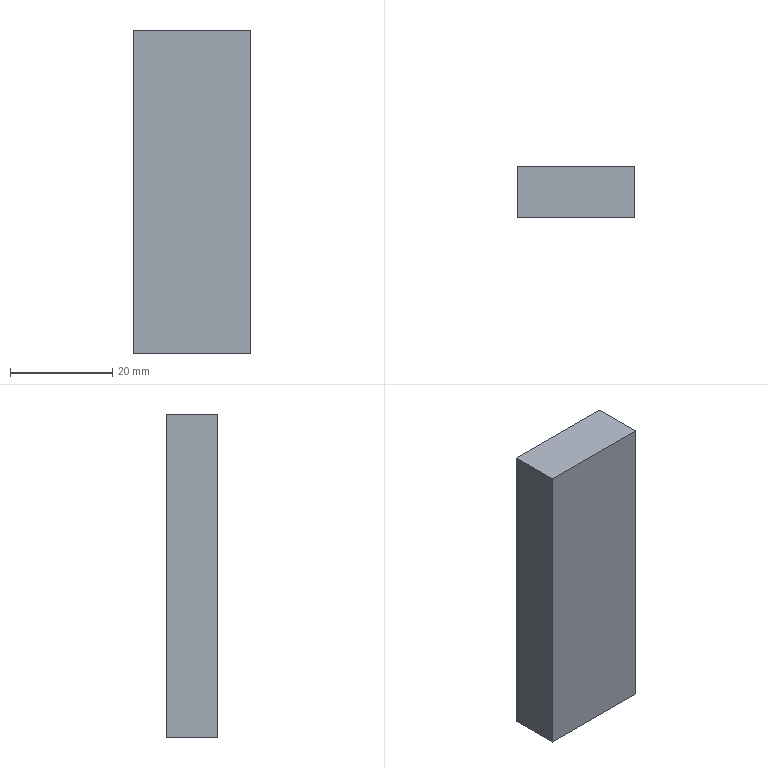Part | SolidWorks | features Extrusion 1 | 1 solid | 6 faces | box 23 x 10 x 63 mm | volume 14490 mm3 | plane 6
STEP:
#1=CARTESIAN_POINT('',(0.,0.,-63.));
#2=VERTEX_POINT('',#1);
#3=CARTESIAN_POINT('',(0.,0.,0.));
#4=VERTEX_POINT('',#3);
#5=CARTESIAN_POINT('',(0.,0.,0.));
#6=DIRECTION('',(0.,0.,1.));
#7=VECTOR('',#6,1000.);
#8=LINE('',#5,#7);
#9=EDGE_CURVE('',#2,#4,#8,.T.);
#10=ORIENTED_EDGE('',*,*,#9,.T.);
#11=CARTESIAN_POINT('',(0.,10.,0.));
#12=VERTEX_POINT('',#11);
#13=CARTESIAN_POINT('',(0.,10.,0.));
#14=DIRECTION('',(0.,-1.,0.));
#15=VECTOR('',#14,1000.);
#16=LINE('',#13,#15);
#17=EDGE_CURVE('',#12,#4,#16,.T.);
#18=ORIENTED_EDGE('',*,*,#17,.F.);
#19=CARTESIAN_POINT('',(0.,10.,-63.));
#20=VERTEX_POINT('',#19);
#21=CARTESIAN_POINT('',(0.,10.,0.));
#22=DIRECTION('',(0.,0.,1.));
#23=VECTOR('',#22,1000.);
#24=LINE('',#21,#23);
#25=EDGE_CURVE('',#20,#12,#24,.T.);
#26=ORIENTED_EDGE('',*,*,#25,.F.);
#27=CARTESIAN_POINT('',(0.,10.,-63.));
#28=DIRECTION('',(0.,-1.,0.));
#29=VECTOR('',#28,1000.);
#30=LINE('',#27,#29);
#31=EDGE_CURVE('',#20,#2,#30,.T.);
#32=ORIENTED_EDGE('',*,*,#31,.T.);
#33=EDGE_LOOP('',(#10,#18,#26,#32));
#34=FACE_OUTER_BOUND('',#33,.T.);
#35=CARTESIAN_POINT('',(0.,10.,0.));
#36=DIRECTION('',(1.,0.,0.));
#37=DIRECTION('',(0.,0.,-1.));
#38=AXIS2_PLACEMENT_3D('',#35,#36,#37);
#39=PLANE('',#38);
#40=ADVANCED_FACE('',(#34),#39,.F.);
#41=CARTESIAN_POINT('',(23.,0.,0.));
#42=VERTEX_POINT('',#41);
#43=CARTESIAN_POINT('',(0.,0.,0.));
#44=DIRECTION('',(1.,0.,0.));
#45=VECTOR('',#44,1000.);
#46=LINE('',#43,#45);
#47=EDGE_CURVE('',#4,#42,#46,.T.);
#48=ORIENTED_EDGE('',*,*,#47,.T.);
#49=CARTESIAN_POINT('',(23.,10.,0.));
#50=VERTEX_POINT('',#49);
#51=CARTESIAN_POINT('',(23.,10.,0.));
#52=DIRECTION('',(0.,-1.,0.));
#53=VECTOR('',#52,1000.);
#54=LINE('',#51,#53);
#55=EDGE_CURVE('',#50,#42,#54,.T.);
#56=ORIENTED_EDGE('',*,*,#55,.F.);
#57=CARTESIAN_POINT('',(0.,10.,0.));
#58=DIRECTION('',(1.,0.,0.));
#59=VECTOR('',#58,1000.);
#60=LINE('',#57,#59);
#61=EDGE_CURVE('',#12,#50,#60,.T.);
#62=ORIENTED_EDGE('',*,*,#61,.F.);
#63=ORIENTED_EDGE('',*,*,#17,.T.);
#64=EDGE_LOOP('',(#48,#56,#62,#63));
#65=FACE_OUTER_BOUND('',#64,.T.);
#66=CARTESIAN_POINT('',(0.,10.,0.));
#67=DIRECTION('',(0.,0.,-1.));
#68=DIRECTION('',(-1.,0.,0.));
#69=AXIS2_PLACEMENT_3D('',#66,#67,#68);
#70=PLANE('',#69);
#71=ADVANCED_FACE('',(#65),#70,.F.);
#72=CARTESIAN_POINT('',(23.,0.,-63.));
#73=VERTEX_POINT('',#72);
#74=CARTESIAN_POINT('',(23.,0.,0.));
#75=DIRECTION('',(0.,0.,-1.));
#76=VECTOR('',#75,1000.);
#77=LINE('',#74,#76);
#78=EDGE_CURVE('',#42,#73,#77,.T.);
#79=ORIENTED_EDGE('',*,*,#78,.T.);
#80=CARTESIAN_POINT('',(23.,10.,-63.));
#81=VERTEX_POINT('',#80);
#82=CARTESIAN_POINT('',(23.,10.,-63.));
#83=DIRECTION('',(0.,-1.,0.));
#84=VECTOR('',#83,1000.);
#85=LINE('',#82,#84);
#86=EDGE_CURVE('',#81,#73,#85,.T.);
#87=ORIENTED_EDGE('',*,*,#86,.F.);
#88=CARTESIAN_POINT('',(23.,10.,0.));
#89=DIRECTION('',(0.,0.,-1.));
#90=VECTOR('',#89,1000.);
#91=LINE('',#88,#90);
#92=EDGE_CURVE('',#50,#81,#91,.T.);
#93=ORIENTED_EDGE('',*,*,#92,.F.);
#94=ORIENTED_EDGE('',*,*,#55,.T.);
#95=EDGE_LOOP('',(#79,#87,#93,#94));
#96=FACE_OUTER_BOUND('',#95,.T.);
#97=CARTESIAN_POINT('',(23.,10.,0.));
#98=DIRECTION('',(-1.,0.,0.));
#99=DIRECTION('',(0.,0.,1.));
#100=AXIS2_PLACEMENT_3D('',#97,#98,#99);
#101=PLANE('',#100);
#102=ADVANCED_FACE('',(#96),#101,.F.);
#103=CARTESIAN_POINT('',(0.,0.,-63.));
#104=DIRECTION('',(-1.,0.,0.));
#105=VECTOR('',#104,1000.);
#106=LINE('',#103,#105);
#107=EDGE_CURVE('',#73,#2,#106,.T.);
#108=ORIENTED_EDGE('',*,*,#107,.T.);
#109=ORIENTED_EDGE('',*,*,#31,.F.);
#110=CARTESIAN_POINT('',(0.,10.,-63.));
#111=DIRECTION('',(-1.,0.,0.));
#112=VECTOR('',#111,1000.);
#113=LINE('',#110,#112);
#114=EDGE_CURVE('',#81,#20,#113,.T.);
#115=ORIENTED_EDGE('',*,*,#114,.F.);
#116=ORIENTED_EDGE('',*,*,#86,.T.);
#117=EDGE_LOOP('',(#108,#109,#115,#116));
#118=FACE_OUTER_BOUND('',#117,.T.);
#119=CARTESIAN_POINT('',(0.,10.,-63.));
#120=DIRECTION('',(0.,0.,1.));
#121=DIRECTION('',(1.,0.,0.));
#122=AXIS2_PLACEMENT_3D('',#119,#120,#121);
#123=PLANE('',#122);
#124=ADVANCED_FACE('',(#118),#123,.F.);
#125=ORIENTED_EDGE('',*,*,#25,.T.);
#126=ORIENTED_EDGE('',*,*,#61,.T.);
#127=ORIENTED_EDGE('',*,*,#92,.T.);
#128=ORIENTED_EDGE('',*,*,#114,.T.);
#129=EDGE_LOOP('',(#125,#126,#127,#128));
#130=FACE_OUTER_BOUND('',#129,.T.);
#131=CARTESIAN_POINT('',(0.,10.,0.));
#132=DIRECTION('',(0.,-1.,0.));
#133=DIRECTION('',(0.,0.,-1.));
#134=AXIS2_PLACEMENT_3D('',#131,#132,#133);
#135=PLANE('',#134);
#136=ADVANCED_FACE('',(#130),#135,.F.);
#137=ORIENTED_EDGE('',*,*,#9,.F.);
#138=ORIENTED_EDGE('',*,*,#107,.F.);
#139=ORIENTED_EDGE('',*,*,#78,.F.);
#140=ORIENTED_EDGE('',*,*,#47,.F.);
#141=EDGE_LOOP('',(#137,#138,#139,#140));
#142=FACE_OUTER_BOUND('',#141,.T.);
#143=CARTESIAN_POINT('',(0.,0.,0.));
#144=DIRECTION('',(0.,-1.,0.));
#145=DIRECTION('',(0.,0.,-1.));
#146=AXIS2_PLACEMENT_3D('',#143,#144,#145);
#147=PLANE('',#146);
#148=ADVANCED_FACE('',(#142),#147,.T.);
#149=CLOSED_SHELL('',(#40,#71,#102,#124,#136,#148));
#150=MANIFOLD_SOLID_BREP('',#149);
#151=CARTESIAN_POINT('',(0.,0.,0.));
#152=DIRECTION('',(0.,0.,1.));
#153=DIRECTION('',(1.,0.,0.));
#154=AXIS2_PLACEMENT_3D('',#151,#152,#153);
#155=(LENGTH_UNIT()NAMED_UNIT(*)SI_UNIT(.MILLI.,.METRE.));
#156=UNCERTAINTY_MEASURE_WITH_UNIT(LENGTH_MEASURE(0.00001),#155,'','');
#157=(NAMED_UNIT(*)PLANE_ANGLE_UNIT()SI_UNIT($,.RADIAN.));
#158=(NAMED_UNIT(*)SI_UNIT($,.STERADIAN.)SOLID_ANGLE_UNIT());
#159=(GEOMETRIC_REPRESENTATION_CONTEXT(3)GLOBAL_UNCERTAINTY_ASSIGNED_CONTEXT((#156))GLOBAL_UNIT_ASSIGNED_CONTEXT((#155,#157,#158))REPRESENTATION_CONTEXT('',''));
#160=ADVANCED_BREP_SHAPE_REPRESENTATION('',(#150,#154),#159);